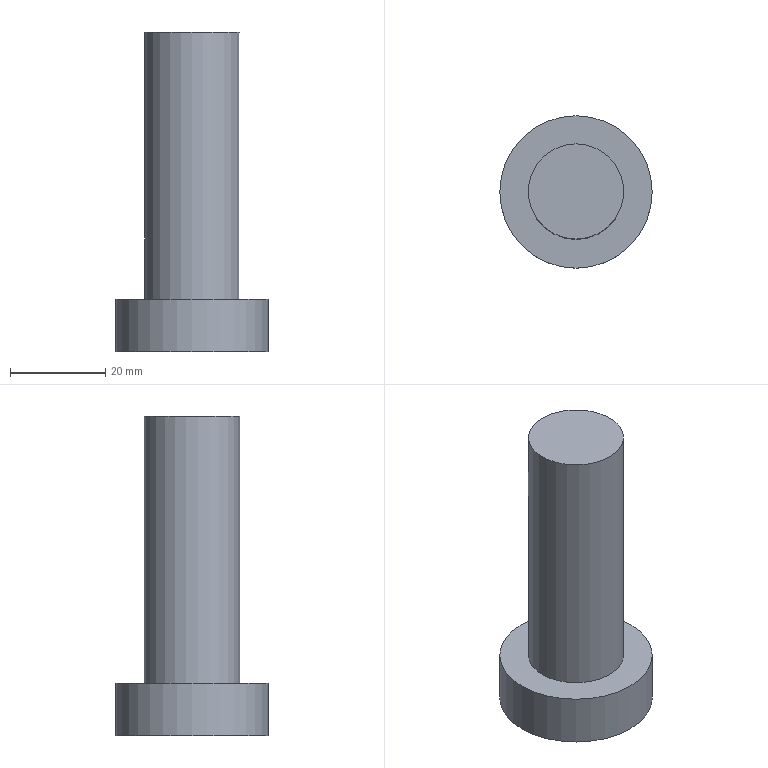Part | NX | features solid 2 | 1 solid | 5 faces | box 32 x 32 x 67 mm | volume 26440 mm3 | plane 3 | cylinder 2 | commonest cylinder face diameters 20 x1 32 x1
STEP:
#1=CARTESIAN_POINT('',(652.5,-124.,-80.));
#2=VERTEX_POINT('',#1);
#3=CARTESIAN_POINT('',(652.5,-140.,-80.));
#4=DIRECTION('',(0.,0.,-1.));
#5=DIRECTION('',(0.,1.,0.));
#6=AXIS2_PLACEMENT_3D('',#3,#4,#5);
#7=CIRCLE('',#6,16.);
#8=EDGE_CURVE('',#2,#2,#7,.T.);
#9=ORIENTED_EDGE('',*,*,#8,.F.);
#10=EDGE_LOOP('',(#9));
#11=FACE_BOUND('',#10,.T.);
#12=CARTESIAN_POINT('',(652.5,-130.,-80.));
#13=VERTEX_POINT('',#12);
#14=CARTESIAN_POINT('',(652.5,-140.,-80.));
#15=DIRECTION('',(0.,0.,-1.));
#16=DIRECTION('',(0.,1.,0.));
#17=AXIS2_PLACEMENT_3D('',#14,#15,#16);
#18=CIRCLE('',#17,10.);
#19=EDGE_CURVE('',#13,#13,#18,.T.);
#20=ORIENTED_EDGE('',*,*,#19,.T.);
#21=EDGE_LOOP('',(#20));
#22=FACE_BOUND('',#21,.T.);
#23=CARTESIAN_POINT('',(652.5,-140.,-80.));
#24=DIRECTION('',(0.,0.,1.));
#25=DIRECTION('',(0.,1.,0.));
#26=AXIS2_PLACEMENT_3D('',#23,#24,#25);
#27=PLANE('',#26);
#28=ADVANCED_FACE('',(#11,#22),#27,.T.);
#29=CARTESIAN_POINT('',(652.5,-124.,-91.));
#30=VERTEX_POINT('',#29);
#31=CARTESIAN_POINT('',(652.5,-140.,-91.));
#32=DIRECTION('',(0.,0.,-1.));
#33=DIRECTION('',(0.,1.,0.));
#34=AXIS2_PLACEMENT_3D('',#31,#32,#33);
#35=CIRCLE('',#34,16.);
#36=EDGE_CURVE('',#30,#30,#35,.T.);
#37=ORIENTED_EDGE('',*,*,#36,.F.);
#38=EDGE_LOOP('',(#37));
#39=FACE_BOUND('',#38,.T.);
#40=ORIENTED_EDGE('',*,*,#8,.T.);
#41=EDGE_LOOP('',(#40));
#42=FACE_BOUND('',#41,.T.);
#43=CARTESIAN_POINT('',(652.5,-140.,-80.));
#44=DIRECTION('',(0.,0.,-1.));
#45=DIRECTION('',(0.,-1.,0.));
#46=AXIS2_PLACEMENT_3D('',#43,#44,#45);
#47=CYLINDRICAL_SURFACE('',#46,16.);
#48=ADVANCED_FACE('',(#39,#42),#47,.T.);
#49=CARTESIAN_POINT('',(652.5,-130.,-24.));
#50=VERTEX_POINT('',#49);
#51=CARTESIAN_POINT('',(652.5,-140.,-24.));
#52=DIRECTION('',(0.,0.,-1.));
#53=DIRECTION('',(0.,1.,0.));
#54=AXIS2_PLACEMENT_3D('',#51,#52,#53);
#55=CIRCLE('',#54,10.);
#56=EDGE_CURVE('',#50,#50,#55,.T.);
#57=ORIENTED_EDGE('',*,*,#56,.T.);
#58=EDGE_LOOP('',(#57));
#59=FACE_BOUND('',#58,.T.);
#60=ORIENTED_EDGE('',*,*,#19,.F.);
#61=EDGE_LOOP('',(#60));
#62=FACE_BOUND('',#61,.T.);
#63=CARTESIAN_POINT('',(652.5,-140.,-24.));
#64=DIRECTION('',(0.,0.,-1.));
#65=DIRECTION('',(0.,-1.,0.));
#66=AXIS2_PLACEMENT_3D('',#63,#64,#65);
#67=CYLINDRICAL_SURFACE('',#66,10.);
#68=ADVANCED_FACE('',(#59,#62),#67,.T.);
#69=ORIENTED_EDGE('',*,*,#56,.F.);
#70=EDGE_LOOP('',(#69));
#71=FACE_BOUND('',#70,.T.);
#72=CARTESIAN_POINT('',(652.5,-210.,-24.));
#73=DIRECTION('',(0.,0.,1.));
#74=DIRECTION('',(0.,1.,0.));
#75=AXIS2_PLACEMENT_3D('',#72,#73,#74);
#76=PLANE('',#75);
#77=ADVANCED_FACE('',(#71),#76,.T.);
#78=ORIENTED_EDGE('',*,*,#36,.T.);
#79=EDGE_LOOP('',(#78));
#80=FACE_BOUND('',#79,.T.);
#81=CARTESIAN_POINT('',(615.,15.,-91.));
#82=DIRECTION('',(0.,0.,1.));
#83=DIRECTION('',(0.,1.,0.));
#84=AXIS2_PLACEMENT_3D('',#81,#82,#83);
#85=PLANE('',#84);
#86=ADVANCED_FACE('',(#80),#85,.F.);
#87=CLOSED_SHELL('',(#28,#48,#68,#77,#86));
#88=MANIFOLD_SOLID_BREP('',#87);
#89=(LENGTH_UNIT()NAMED_UNIT(*)SI_UNIT(.MILLI.,.METRE.));
#90=UNCERTAINTY_MEASURE_WITH_UNIT(LENGTH_MEASURE(0.00001),#89,'','');
#91=(NAMED_UNIT(*)PLANE_ANGLE_UNIT()SI_UNIT($,.RADIAN.));
#92=(NAMED_UNIT(*)SI_UNIT($,.STERADIAN.)SOLID_ANGLE_UNIT());
#93=(GEOMETRIC_REPRESENTATION_CONTEXT(3)GLOBAL_UNCERTAINTY_ASSIGNED_CONTEXT((#90))GLOBAL_UNIT_ASSIGNED_CONTEXT((#89,#91,#92))REPRESENTATION_CONTEXT('',''));
#94=ADVANCED_BREP_SHAPE_REPRESENTATION('',(#88),#93);